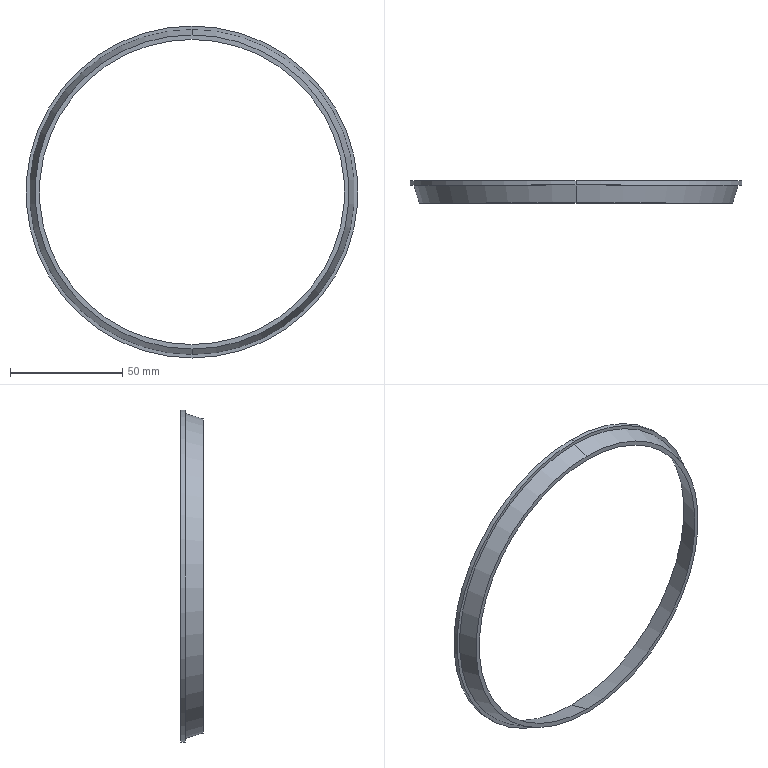Part | SolidWorks | features Revolution 1 | 1 solid | 9 faces | box 148 x 10 x 148 mm | volume 10057 mm3 | cone 4 | plane 3 | cylinder 2 | commonest cylinder face diameters 148 x2
STEP:
#1=CARTESIAN_POINT('',(0.,0.,-70.));
#2=VERTEX_POINT('',#1);
#3=CARTESIAN_POINT('',(0.,0.,70.));
#4=VERTEX_POINT('',#3);
#5=CARTESIAN_POINT('',(0.,0.,0.));
#6=DIRECTION('',(0.,-1.,0.));
#7=DIRECTION('',(0.,0.,-1.));
#8=AXIS2_PLACEMENT_3D('',#5,#6,#7);
#9=CIRCLE('',#8,70.);
#10=EDGE_CURVE('',#2,#4,#9,.T.);
#11=ORIENTED_EDGE('',*,*,#10,.F.);
#12=CARTESIAN_POINT('',(0.,8.,-72.4));
#13=VERTEX_POINT('',#12);
#14=CARTESIAN_POINT('',(0.,8.,-72.4));
#15=DIRECTION('',(0.,0.9578,-0.2873));
#16=VECTOR('',#15,1000.);
#17=LINE('',#14,#16);
#18=EDGE_CURVE('',#2,#13,#17,.T.);
#19=ORIENTED_EDGE('',*,*,#18,.T.);
#20=CARTESIAN_POINT('',(0.,8.,72.4));
#21=VERTEX_POINT('',#20);
#22=CARTESIAN_POINT('',(0.,8.,0.));
#23=DIRECTION('',(0.,-1.,0.));
#24=DIRECTION('',(0.,0.,-1.));
#25=AXIS2_PLACEMENT_3D('',#22,#23,#24);
#26=CIRCLE('',#25,72.4);
#27=EDGE_CURVE('',#13,#21,#26,.T.);
#28=ORIENTED_EDGE('',*,*,#27,.T.);
#29=CARTESIAN_POINT('',(0.,8.,72.4));
#30=DIRECTION('',(0.,0.9578,0.2873));
#31=VECTOR('',#30,1000.);
#32=LINE('',#29,#31);
#33=EDGE_CURVE('',#4,#21,#32,.T.);
#34=ORIENTED_EDGE('',*,*,#33,.F.);
#35=EDGE_LOOP('',(#11,#19,#28,#34));
#36=FACE_OUTER_BOUND('',#35,.T.);
#37=CARTESIAN_POINT('',(0.,8.,0.));
#38=DIRECTION('',(0.,1.,0.));
#39=DIRECTION('',(0.,0.,1.));
#40=AXIS2_PLACEMENT_3D('',#37,#38,#39);
#41=CONICAL_SURFACE('',#40,72.4,0.2915);
#42=ADVANCED_FACE('',(#36),#41,.T.);
#43=CARTESIAN_POINT('',(0.,10.,-74.));
#44=VERTEX_POINT('',#43);
#45=CARTESIAN_POINT('',(0.,10.,74.));
#46=VERTEX_POINT('',#45);
#47=CARTESIAN_POINT('',(0.,10.,0.));
#48=DIRECTION('',(0.,-1.,0.));
#49=DIRECTION('',(0.,0.,-1.));
#50=AXIS2_PLACEMENT_3D('',#47,#48,#49);
#51=CIRCLE('',#50,74.);
#52=EDGE_CURVE('',#44,#46,#51,.T.);
#53=ORIENTED_EDGE('',*,*,#52,.T.);
#54=CARTESIAN_POINT('',(0.,8.,74.));
#55=VERTEX_POINT('',#54);
#56=CARTESIAN_POINT('',(0.,0.,74.));
#57=DIRECTION('',(0.,-1.,0.));
#58=VECTOR('',#57,1000.);
#59=LINE('',#56,#58);
#60=EDGE_CURVE('',#46,#55,#59,.T.);
#61=ORIENTED_EDGE('',*,*,#60,.T.);
#62=CARTESIAN_POINT('',(0.,8.,-74.));
#63=VERTEX_POINT('',#62);
#64=CARTESIAN_POINT('',(0.,8.,0.));
#65=DIRECTION('',(0.,-1.,0.));
#66=DIRECTION('',(0.,0.,-1.));
#67=AXIS2_PLACEMENT_3D('',#64,#65,#66);
#68=CIRCLE('',#67,74.);
#69=EDGE_CURVE('',#63,#55,#68,.T.);
#70=ORIENTED_EDGE('',*,*,#69,.F.);
#71=CARTESIAN_POINT('',(0.,0.,-74.));
#72=DIRECTION('',(0.,-1.,0.));
#73=VECTOR('',#72,1000.);
#74=LINE('',#71,#73);
#75=EDGE_CURVE('',#44,#63,#74,.T.);
#76=ORIENTED_EDGE('',*,*,#75,.F.);
#77=EDGE_LOOP('',(#53,#61,#70,#76));
#78=FACE_OUTER_BOUND('',#77,.T.);
#79=CARTESIAN_POINT('',(0.,0.,0.));
#80=DIRECTION('',(0.,-1.,0.));
#81=DIRECTION('',(0.,0.,-1.));
#82=AXIS2_PLACEMENT_3D('',#79,#80,#81);
#83=CYLINDRICAL_SURFACE('',#82,74.);
#84=ADVANCED_FACE('',(#78),#83,.T.);
#85=CARTESIAN_POINT('',(0.,0.,68.));
#86=VERTEX_POINT('',#85);
#87=CARTESIAN_POINT('',(0.,0.,-68.));
#88=VERTEX_POINT('',#87);
#89=CARTESIAN_POINT('',(0.,0.,0.));
#90=DIRECTION('',(0.,-1.,0.));
#91=DIRECTION('',(0.,0.,-1.));
#92=AXIS2_PLACEMENT_3D('',#89,#90,#91);
#93=CIRCLE('',#92,68.);
#94=EDGE_CURVE('',#86,#88,#93,.T.);
#95=ORIENTED_EDGE('',*,*,#94,.T.);
#96=CARTESIAN_POINT('',(0.,10.,-71.));
#97=VERTEX_POINT('',#96);
#98=CARTESIAN_POINT('',(0.,0.,-68.));
#99=DIRECTION('',(0.,0.9578,-0.2873));
#100=VECTOR('',#99,1000.);
#101=LINE('',#98,#100);
#102=EDGE_CURVE('',#88,#97,#101,.T.);
#103=ORIENTED_EDGE('',*,*,#102,.T.);
#104=CARTESIAN_POINT('',(0.,10.,71.));
#105=VERTEX_POINT('',#104);
#106=CARTESIAN_POINT('',(0.,10.,0.));
#107=DIRECTION('',(0.,-1.,0.));
#108=DIRECTION('',(0.,0.,-1.));
#109=AXIS2_PLACEMENT_3D('',#106,#107,#108);
#110=CIRCLE('',#109,71.);
#111=EDGE_CURVE('',#105,#97,#110,.T.);
#112=ORIENTED_EDGE('',*,*,#111,.F.);
#113=CARTESIAN_POINT('',(0.,0.,68.));
#114=DIRECTION('',(0.,0.9578,0.2873));
#115=VECTOR('',#114,1000.);
#116=LINE('',#113,#115);
#117=EDGE_CURVE('',#86,#105,#116,.T.);
#118=ORIENTED_EDGE('',*,*,#117,.F.);
#119=EDGE_LOOP('',(#95,#103,#112,#118));
#120=FACE_OUTER_BOUND('',#119,.T.);
#121=CARTESIAN_POINT('',(0.,0.,0.));
#122=DIRECTION('',(0.,1.,0.));
#123=DIRECTION('',(0.,0.,1.));
#124=AXIS2_PLACEMENT_3D('',#121,#122,#123);
#125=CONICAL_SURFACE('',#124,68.,0.2915);
#126=ADVANCED_FACE('',(#120),#125,.F.);
#127=ORIENTED_EDGE('',*,*,#102,.F.);
#128=CARTESIAN_POINT('',(0.,0.,0.));
#129=DIRECTION('',(0.,-1.,0.));
#130=DIRECTION('',(0.,0.,-1.));
#131=AXIS2_PLACEMENT_3D('',#128,#129,#130);
#132=CIRCLE('',#131,68.);
#133=EDGE_CURVE('',#88,#86,#132,.T.);
#134=ORIENTED_EDGE('',*,*,#133,.T.);
#135=ORIENTED_EDGE('',*,*,#117,.T.);
#136=CARTESIAN_POINT('',(0.,10.,0.));
#137=DIRECTION('',(0.,-1.,0.));
#138=DIRECTION('',(0.,0.,-1.));
#139=AXIS2_PLACEMENT_3D('',#136,#137,#138);
#140=CIRCLE('',#139,71.);
#141=EDGE_CURVE('',#97,#105,#140,.T.);
#142=ORIENTED_EDGE('',*,*,#141,.F.);
#143=EDGE_LOOP('',(#127,#134,#135,#142));
#144=FACE_OUTER_BOUND('',#143,.T.);
#145=CARTESIAN_POINT('',(0.,0.,0.));
#146=DIRECTION('',(0.,1.,0.));
#147=DIRECTION('',(0.,0.,1.));
#148=AXIS2_PLACEMENT_3D('',#145,#146,#147);
#149=CONICAL_SURFACE('',#148,68.,0.2915);
#150=ADVANCED_FACE('',(#144),#149,.F.);
#151=ORIENTED_EDGE('',*,*,#52,.F.);
#152=CARTESIAN_POINT('',(0.,10.,0.));
#153=DIRECTION('',(0.,-1.,0.));
#154=DIRECTION('',(0.,0.,-1.));
#155=AXIS2_PLACEMENT_3D('',#152,#153,#154);
#156=CIRCLE('',#155,74.);
#157=EDGE_CURVE('',#46,#44,#156,.T.);
#158=ORIENTED_EDGE('',*,*,#157,.F.);
#159=EDGE_LOOP('',(#151,#158));
#160=FACE_OUTER_BOUND('',#159,.T.);
#161=ORIENTED_EDGE('',*,*,#111,.T.);
#162=ORIENTED_EDGE('',*,*,#141,.T.);
#163=EDGE_LOOP('',(#161,#162));
#164=FACE_BOUND('',#163,.T.);
#165=CARTESIAN_POINT('',(0.,10.,0.));
#166=DIRECTION('',(0.,-1.,0.));
#167=DIRECTION('',(0.,0.,-1.));
#168=AXIS2_PLACEMENT_3D('',#165,#166,#167);
#169=PLANE('',#168);
#170=ADVANCED_FACE('',(#160,#164),#169,.F.);
#171=ORIENTED_EDGE('',*,*,#60,.F.);
#172=ORIENTED_EDGE('',*,*,#157,.T.);
#173=ORIENTED_EDGE('',*,*,#75,.T.);
#174=CARTESIAN_POINT('',(0.,8.,0.));
#175=DIRECTION('',(0.,-1.,0.));
#176=DIRECTION('',(0.,0.,-1.));
#177=AXIS2_PLACEMENT_3D('',#174,#175,#176);
#178=CIRCLE('',#177,74.);
#179=EDGE_CURVE('',#55,#63,#178,.T.);
#180=ORIENTED_EDGE('',*,*,#179,.F.);
#181=EDGE_LOOP('',(#171,#172,#173,#180));
#182=FACE_OUTER_BOUND('',#181,.T.);
#183=CARTESIAN_POINT('',(0.,0.,0.));
#184=DIRECTION('',(0.,-1.,0.));
#185=DIRECTION('',(0.,0.,-1.));
#186=AXIS2_PLACEMENT_3D('',#183,#184,#185);
#187=CYLINDRICAL_SURFACE('',#186,74.);
#188=ADVANCED_FACE('',(#182),#187,.T.);
#189=CARTESIAN_POINT('',(0.,8.,0.));
#190=DIRECTION('',(0.,-1.,0.));
#191=DIRECTION('',(0.,0.,-1.));
#192=AXIS2_PLACEMENT_3D('',#189,#190,#191);
#193=CIRCLE('',#192,72.4);
#194=EDGE_CURVE('',#21,#13,#193,.T.);
#195=ORIENTED_EDGE('',*,*,#194,.F.);
#196=ORIENTED_EDGE('',*,*,#27,.F.);
#197=EDGE_LOOP('',(#195,#196));
#198=FACE_BOUND('',#197,.T.);
#199=ORIENTED_EDGE('',*,*,#69,.T.);
#200=ORIENTED_EDGE('',*,*,#179,.T.);
#201=EDGE_LOOP('',(#199,#200));
#202=FACE_OUTER_BOUND('',#201,.T.);
#203=CARTESIAN_POINT('',(0.,8.,0.));
#204=DIRECTION('',(0.,1.,0.));
#205=DIRECTION('',(0.,0.,1.));
#206=AXIS2_PLACEMENT_3D('',#203,#204,#205);
#207=PLANE('',#206);
#208=ADVANCED_FACE('',(#198,#202),#207,.F.);
#209=ORIENTED_EDGE('',*,*,#18,.F.);
#210=CARTESIAN_POINT('',(0.,0.,0.));
#211=DIRECTION('',(0.,-1.,0.));
#212=DIRECTION('',(0.,0.,-1.));
#213=AXIS2_PLACEMENT_3D('',#210,#211,#212);
#214=CIRCLE('',#213,70.);
#215=EDGE_CURVE('',#4,#2,#214,.T.);
#216=ORIENTED_EDGE('',*,*,#215,.F.);
#217=ORIENTED_EDGE('',*,*,#33,.T.);
#218=ORIENTED_EDGE('',*,*,#194,.T.);
#219=EDGE_LOOP('',(#209,#216,#217,#218));
#220=FACE_OUTER_BOUND('',#219,.T.);
#221=CARTESIAN_POINT('',(0.,8.,0.));
#222=DIRECTION('',(0.,1.,0.));
#223=DIRECTION('',(0.,0.,1.));
#224=AXIS2_PLACEMENT_3D('',#221,#222,#223);
#225=CONICAL_SURFACE('',#224,72.4,0.2915);
#226=ADVANCED_FACE('',(#220),#225,.T.);
#227=ORIENTED_EDGE('',*,*,#94,.F.);
#228=ORIENTED_EDGE('',*,*,#133,.F.);
#229=EDGE_LOOP('',(#227,#228));
#230=FACE_BOUND('',#229,.T.);
#231=ORIENTED_EDGE('',*,*,#215,.T.);
#232=ORIENTED_EDGE('',*,*,#10,.T.);
#233=EDGE_LOOP('',(#231,#232));
#234=FACE_OUTER_BOUND('',#233,.T.);
#235=CARTESIAN_POINT('',(0.,0.,0.));
#236=DIRECTION('',(0.,1.,0.));
#237=DIRECTION('',(0.,0.,1.));
#238=AXIS2_PLACEMENT_3D('',#235,#236,#237);
#239=PLANE('',#238);
#240=ADVANCED_FACE('',(#230,#234),#239,.F.);
#241=CLOSED_SHELL('',(#42,#84,#126,#150,#170,#188,#208,#226,#240));
#242=MANIFOLD_SOLID_BREP('',#241);
#243=CARTESIAN_POINT('',(0.,0.,0.));
#244=DIRECTION('',(0.,0.,1.));
#245=DIRECTION('',(1.,0.,0.));
#246=AXIS2_PLACEMENT_3D('',#243,#244,#245);
#247=(LENGTH_UNIT()NAMED_UNIT(*)SI_UNIT(.MILLI.,.METRE.));
#248=UNCERTAINTY_MEASURE_WITH_UNIT(LENGTH_MEASURE(0.00001),#247,'','');
#249=(NAMED_UNIT(*)PLANE_ANGLE_UNIT()SI_UNIT($,.RADIAN.));
#250=(NAMED_UNIT(*)SI_UNIT($,.STERADIAN.)SOLID_ANGLE_UNIT());
#251=(GEOMETRIC_REPRESENTATION_CONTEXT(3)GLOBAL_UNCERTAINTY_ASSIGNED_CONTEXT((#248))GLOBAL_UNIT_ASSIGNED_CONTEXT((#247,#249,#250))REPRESENTATION_CONTEXT('',''));
#252=ADVANCED_BREP_SHAPE_REPRESENTATION('',(#242,#246),#251);